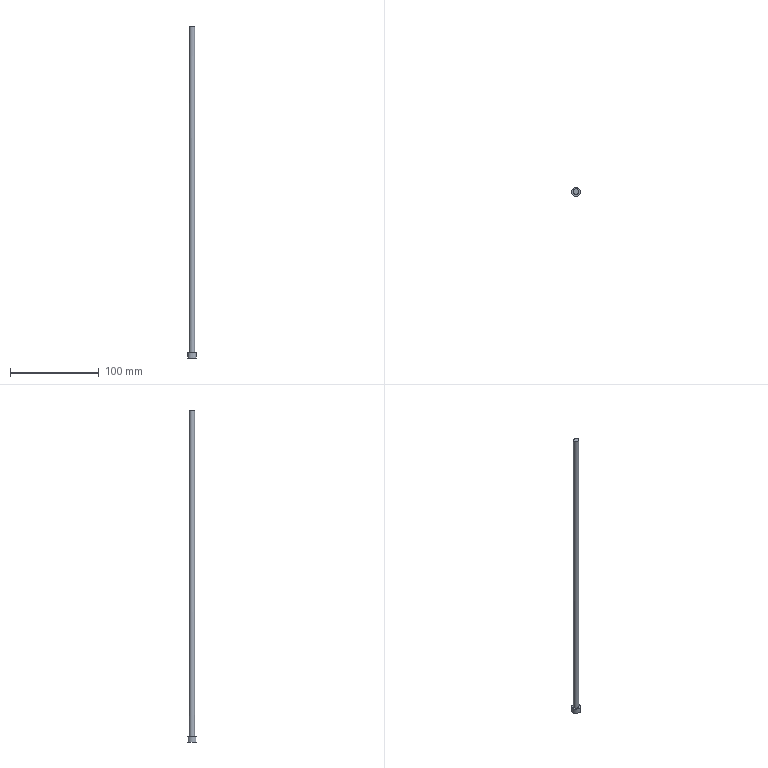Part | NX | features solid 2 | 1 solid | 5 faces | box 10 x 10 x 373.555 mm | volume 10849 mm3 | cylinder 2 | plane 2 | spline 1 | commonest cylinder face diameters 6 x1 10 x1
STEP:
#1=CARTESIAN_POINT('',(56.,31.,-339.5));
#2=VERTEX_POINT('',#1);
#3=CARTESIAN_POINT('',(59.,31.,-339.5));
#4=DIRECTION('',(0.,0.,1.));
#5=DIRECTION('',(-1.,0.,0.));
#6=AXIS2_PLACEMENT_3D('',#3,#4,#5);
#7=CIRCLE('',#6,3.);
#8=EDGE_CURVE('',#2,#2,#7,.T.);
#9=ORIENTED_EDGE('',*,*,#8,.T.);
#10=EDGE_LOOP('',(#9));
#11=FACE_BOUND('',#10,.T.);
#12=CARTESIAN_POINT('',(56.016,30.69,27.216));
#13=VERTEX_POINT('',#12);
#14=CARTESIAN_POINT('',(56.915,28.413,27.375));
#15=CARTESIAN_POINT('',(55.689,30.654,27.171));
#16=CARTESIAN_POINT('',(56.428,33.108,27.239));
#17=CARTESIAN_POINT('',(58.663,34.303,27.536));
#18=CARTESIAN_POINT('',(61.087,33.586,27.887));
#19=CARTESIAN_POINT('',(62.31,31.347,28.092));
#20=CARTESIAN_POINT('',(61.576,28.895,28.023));
#21=CARTESIAN_POINT('',(59.337,27.697,27.725));
#22=CARTESIAN_POINT('',(56.915,28.413,27.375));
#23=CARTESIAN_POINT('',(55.689,30.654,27.171));
#24=CARTESIAN_POINT('',(56.428,33.108,27.239));
#25=B_SPLINE_CURVE_WITH_KNOTS('',3,(#14,#15,#16,#17,#18,#19,#20,#21,#22,#23,#24),.UNSPECIFIED.,.T.,.F.,(1,1,1,1,1,1,1,1,1,1,1,1,1,1,1),(-0.00707,-0.004713,-0.002357,0.,0.002357,0.004713,0.00707,0.009426,0.01178,0.01414,0.0165,0.01885,0.02121,0.02357,0.02592),.UNSPECIFIED.);
#26=EDGE_CURVE('',#13,#13,#25,.T.);
#27=ORIENTED_EDGE('',*,*,#26,.T.);
#28=EDGE_LOOP('',(#27));
#29=FACE_BOUND('',#28,.T.);
#30=CARTESIAN_POINT('',(59.,31.,-345.5));
#31=DIRECTION('',(0.,0.,1.));
#32=DIRECTION('',(-1.,0.,0.));
#33=AXIS2_PLACEMENT_3D('',#30,#31,#32);
#34=CYLINDRICAL_SURFACE('',#33,3.);
#35=ADVANCED_FACE('',(#11,#29),#34,.T.);
#36=ORIENTED_EDGE('',*,*,#8,.F.);
#37=EDGE_LOOP('',(#36));
#38=FACE_BOUND('',#37,.T.);
#39=CARTESIAN_POINT('',(54.,31.,-339.5));
#40=VERTEX_POINT('',#39);
#41=CARTESIAN_POINT('',(59.,31.,-339.5));
#42=DIRECTION('',(0.,0.,-1.));
#43=DIRECTION('',(-1.,0.,0.));
#44=AXIS2_PLACEMENT_3D('',#41,#42,#43);
#45=CIRCLE('',#44,5.);
#46=EDGE_CURVE('',#40,#40,#45,.T.);
#47=ORIENTED_EDGE('',*,*,#46,.F.);
#48=EDGE_LOOP('',(#47));
#49=FACE_BOUND('',#48,.T.);
#50=CARTESIAN_POINT('',(59.,31.,-339.5));
#51=DIRECTION('',(0.,0.,1.));
#52=DIRECTION('',(-1.,0.,0.));
#53=AXIS2_PLACEMENT_3D('',#50,#51,#52);
#54=PLANE('',#53);
#55=ADVANCED_FACE('',(#38,#49),#54,.T.);
#56=CARTESIAN_POINT('',(54.,31.,-345.5));
#57=VERTEX_POINT('',#56);
#58=CARTESIAN_POINT('',(59.,31.,-345.5));
#59=DIRECTION('',(0.,0.,1.));
#60=DIRECTION('',(-1.,0.,0.));
#61=AXIS2_PLACEMENT_3D('',#58,#59,#60);
#62=CIRCLE('',#61,5.);
#63=EDGE_CURVE('',#57,#57,#62,.T.);
#64=ORIENTED_EDGE('',*,*,#63,.F.);
#65=EDGE_LOOP('',(#64));
#66=FACE_BOUND('',#65,.T.);
#67=CARTESIAN_POINT('',(59.,31.,-345.5));
#68=DIRECTION('',(0.,0.,-1.));
#69=DIRECTION('',(1.,0.,0.));
#70=AXIS2_PLACEMENT_3D('',#67,#68,#69);
#71=PLANE('',#70);
#72=ADVANCED_FACE('',(#66),#71,.T.);
#73=ORIENTED_EDGE('',*,*,#46,.T.);
#74=EDGE_LOOP('',(#73));
#75=FACE_BOUND('',#74,.T.);
#76=ORIENTED_EDGE('',*,*,#63,.T.);
#77=EDGE_LOOP('',(#76));
#78=FACE_BOUND('',#77,.T.);
#79=CARTESIAN_POINT('',(59.,31.,-345.5));
#80=DIRECTION('',(0.,0.,1.));
#81=DIRECTION('',(-1.,0.,0.));
#82=AXIS2_PLACEMENT_3D('',#79,#80,#81);
#83=CYLINDRICAL_SURFACE('',#82,5.);
#84=ADVANCED_FACE('',(#75,#78),#83,.T.);
#85=ORIENTED_EDGE('',*,*,#26,.F.);
#86=EDGE_LOOP('',(#85));
#87=FACE_BOUND('',#86,.T.);
#88=CARTESIAN_POINT('',(55.943,27.944,27.244));
#89=CARTESIAN_POINT('',(55.945,29.974,27.217));
#90=CARTESIAN_POINT('',(55.946,32.005,27.188));
#91=CARTESIAN_POINT('',(55.948,34.036,27.158));
#92=CARTESIAN_POINT('',(57.979,27.945,27.531));
#93=CARTESIAN_POINT('',(57.981,29.975,27.504));
#94=CARTESIAN_POINT('',(57.982,32.005,27.475));
#95=CARTESIAN_POINT('',(57.984,34.036,27.445));
#96=CARTESIAN_POINT('',(60.016,27.945,27.817));
#97=CARTESIAN_POINT('',(60.017,29.976,27.79));
#98=CARTESIAN_POINT('',(60.019,32.006,27.761));
#99=CARTESIAN_POINT('',(60.02,34.037,27.731));
#100=CARTESIAN_POINT('',(62.052,27.946,28.103));
#101=CARTESIAN_POINT('',(62.054,29.976,28.076));
#102=CARTESIAN_POINT('',(62.055,32.007,28.047));
#103=CARTESIAN_POINT('',(62.057,34.037,28.017));
#104=B_SPLINE_SURFACE_WITH_KNOTS('',3,3,((#88,#89,#90,#91),(#92,#93,#94,#95),(#96,#97,#98,#99),(#100,#101,#102,#103)),.UNSPECIFIED.,.F.,.F.,.F.,(4,4),(4,4),(0.9324,0.9631),(0.08216,0.1978),.PIECEWISE_BEZIER_KNOTS.);
#105=ADVANCED_FACE('',(#87),#104,.T.);
#106=CLOSED_SHELL('',(#35,#55,#72,#84,#105));
#107=MANIFOLD_SOLID_BREP('',#106);
#108=(LENGTH_UNIT()NAMED_UNIT(*)SI_UNIT(.MILLI.,.METRE.));
#109=UNCERTAINTY_MEASURE_WITH_UNIT(LENGTH_MEASURE(0.0508),#108,'','');
#110=(NAMED_UNIT(*)PLANE_ANGLE_UNIT()SI_UNIT($,.RADIAN.));
#111=(NAMED_UNIT(*)SI_UNIT($,.STERADIAN.)SOLID_ANGLE_UNIT());
#112=(GEOMETRIC_REPRESENTATION_CONTEXT(3)GLOBAL_UNCERTAINTY_ASSIGNED_CONTEXT((#109))GLOBAL_UNIT_ASSIGNED_CONTEXT((#108,#110,#111))REPRESENTATION_CONTEXT('',''));
#113=ADVANCED_BREP_SHAPE_REPRESENTATION('',(#107),#112);